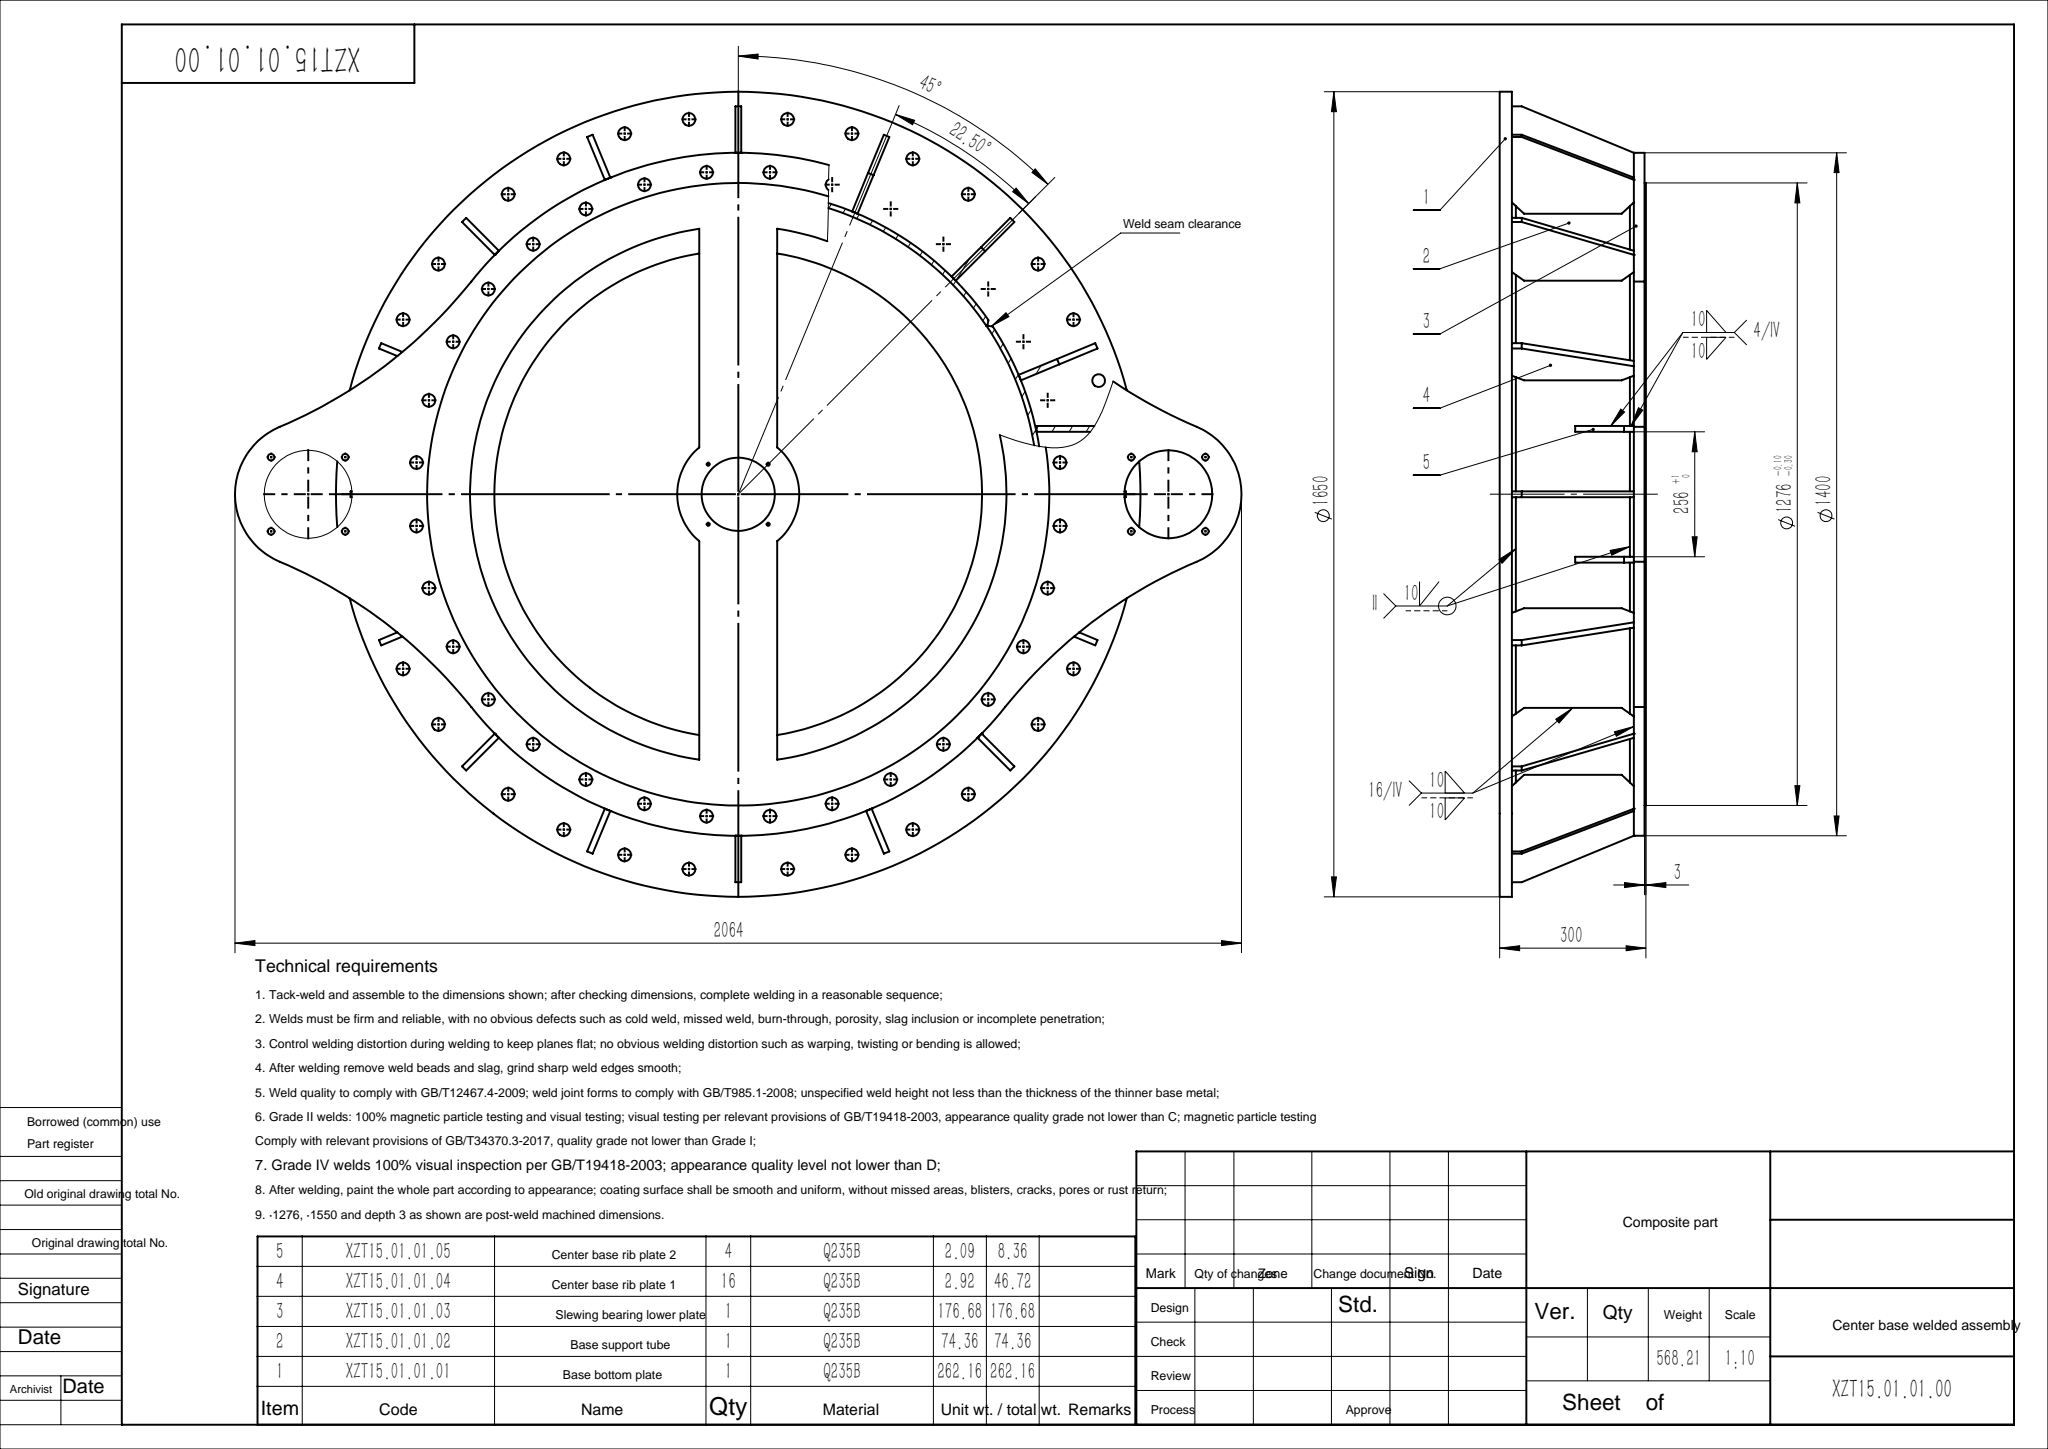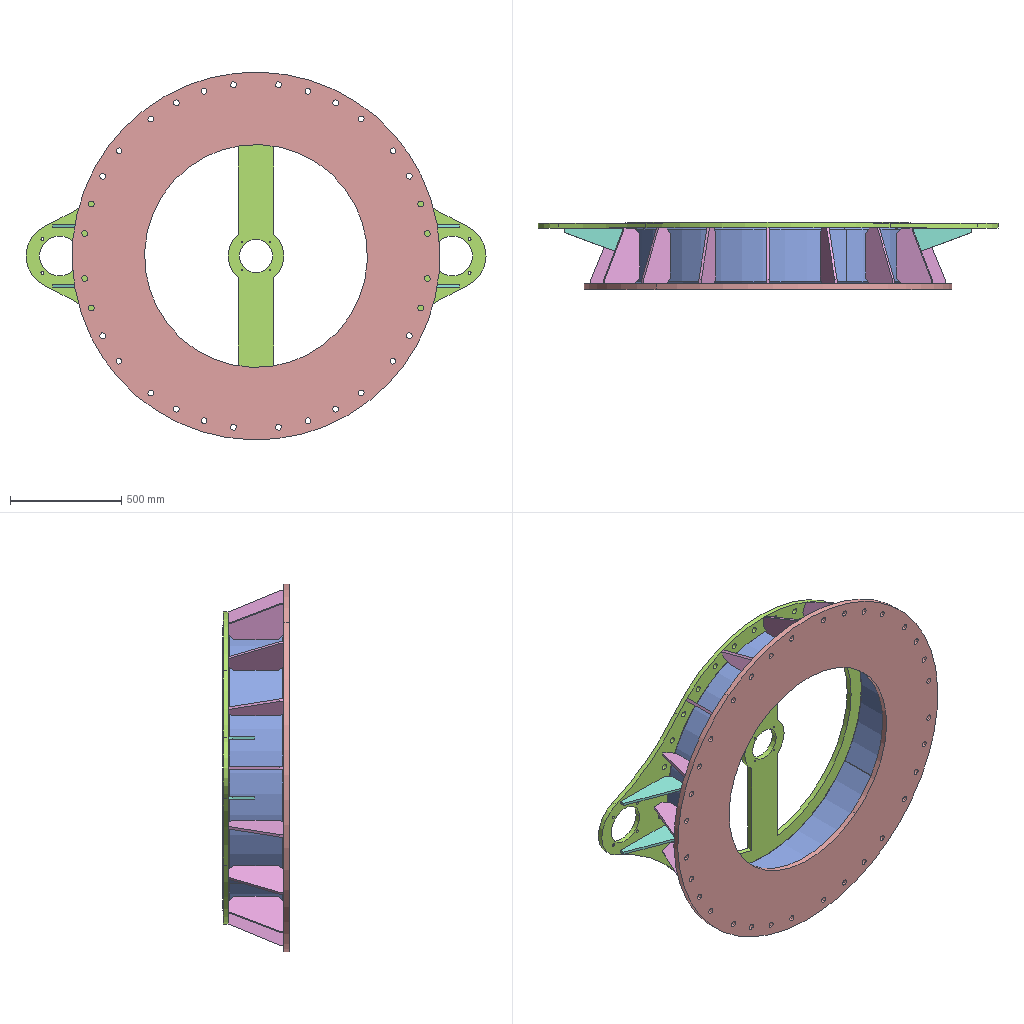Assembly | SolidWorks | 5 different items | 23 placed | box 2064 x 300 x 1649 mm
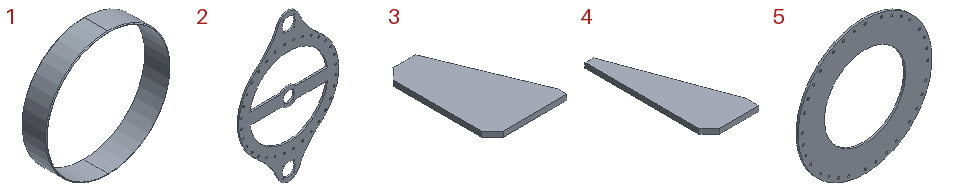Parts list (item | quantity | size | volume | features):
1 | x1 | 1250 x 250 x 1250 mm | 9472946 mm3 | features Chamfer 2, FlatPattern 1, SMBaseFlange 1, SheetMetal 1
2 | x1 | 1400 x 25 x 2064 mm | 22506945 mm3 | features HoleWzd 3, Extrusion 1, ICE 1, MirrorPattern 1
3 | x16 | 170 x 250 x 12 mm | 371400 mm3 | features Chamfer 1, Extrusion 1
4 | x4 | 120 x 300 x 12 mm | 266250 mm3 | features Chamfer 1, Extrusion 1
5 | x1 | 1650 x 25 x 1650 mm | 33396465 mm3 | features Extrusion 1, HoleWzd 1
Mates (type | each side: item.copy, entity, surface, feature):
Concentric | assembly axis | 5.1 face cylinder Boss-Extrude1
Concentric | assembly axis | 1.1 face cylinder Base-Bend1
Concentric | assembly axis | 2.1 face cylinder Boss-Extrude1
PlanarAngleDim | assembly plane | 5.1 plane
Coincident | 5.1 face plane Boss-Extrude1 | 1.1 face plane Base-Bend1
Coincident | 1.1 face plane Base-Bend1 | 2.1 face plane Boss-Extrude1
Coincident | 2.1 plane | assembly plane
Coincident | 5.1 face plane Boss-Extrude1 | 3.1 face plane Boss-Extrude1
Coincident | 5.1 face plane Boss-Extrude1 | assembly plane
Coincident | 3.1 plane | assembly plane
Tangent | 1.1 face cylinder Base-Bend1 | 3.1 face plane Boss-Extrude1
Coincident | 2.1 face plane Boss-Extrude1 | 4.1 face plane Boss-Extrude1
DistanceDim | 4.1 face plane Boss-Extrude1 | 4.2 face plane Boss-Extrude1
Coincident | 1.1 face cylinder Base-Bend1 | 4.1 edge